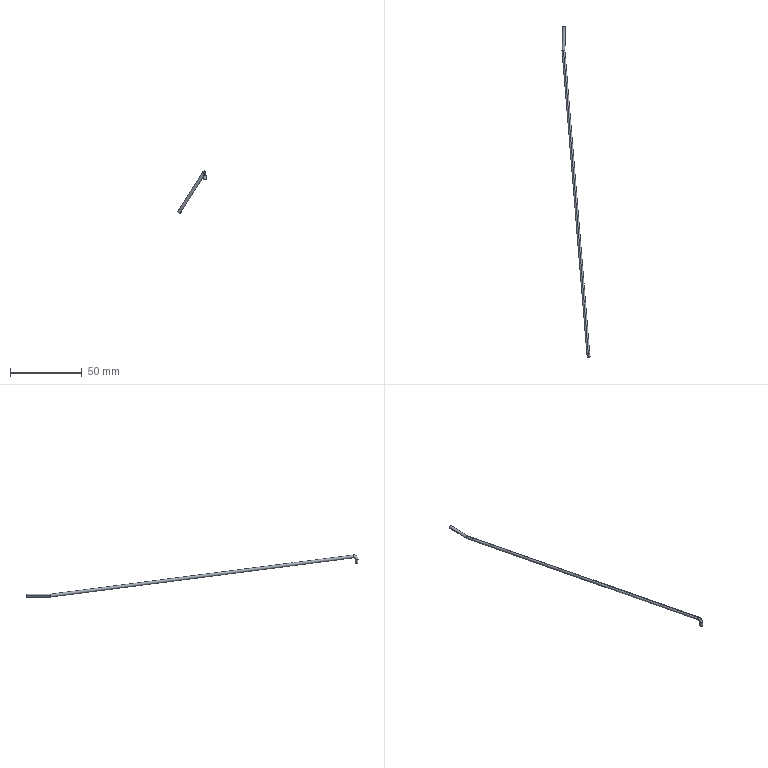Part | STEP file | rear_spoke4 | 1 solid | 10 faces | box 19.566 x 231.981 x 29.396 mm | volume 746.049 mm3 | cylinder 6 | torus 2 | plane 2 | commonest cylinder face diameters 2 x6
STEP:
#1=CARTESIAN_POINT('',(0.,0.,0.));
#2=DIRECTION('',(0.,0.,1.));
#3=DIRECTION('',(1.,0.,0.));
#4=AXIS2_PLACEMENT_3D('',#1,#2,#3);
#5=CARTESIAN_POINT('',(23.113,16.112,-0.1044));
#6=VERTEX_POINT('',#5);
#7=CARTESIAN_POINT('',(24.194,15.115,-0.1044));
#8=VERTEX_POINT('',#7);
#9=CARTESIAN_POINT('',(24.113,16.112,-0.1044));
#10=DIRECTION('',(0.,0.,1.));
#11=DIRECTION('',(1.,0.,0.));
#12=AXIS2_PLACEMENT_3D('',#9,#10,#11);
#13=CIRCLE('',#12,1.);
#14=CARTESIAN_POINT('',(23.949,18.105,-0.1044));
#15=DIRECTION('',(-0.9966,-0.08183,0.));
#16=DIRECTION('',(0.08183,-0.9966,0.));
#17=AXIS2_PLACEMENT_3D('',#14,#15,#16);
#18=TOROIDAL_SURFACE('',#17,2.,1.);
#19=CARTESIAN_POINT('',(0.,4.794));
#20=DIRECTION('',(0.,-1.));
#21=VECTOR('',#20,1.);
#22=LINE('',#19,#21);
#23=(GEOMETRIC_REPRESENTATION_CONTEXT(2)PARAMETRIC_REPRESENTATION_CONTEXT()REPRESENTATION_CONTEXT('',''));
#24=DEFINITIONAL_REPRESENTATION('',(#22),#23);
#25=PCURVE('',#18,#24);
#26=CARTESIAN_POINT('',(24.113,16.112,-3.));
#27=DIRECTION('',(0.,0.,1.));
#28=DIRECTION('',(1.,0.,0.));
#29=AXIS2_PLACEMENT_3D('',#26,#27,#28);
#30=CYLINDRICAL_SURFACE('',#29,1.);
#31=CARTESIAN_POINT('',(0.,2.896));
#32=DIRECTION('',(1.,0.));
#33=VECTOR('',#32,1.);
#34=LINE('',#31,#33);
#35=(GEOMETRIC_REPRESENTATION_CONTEXT(2)PARAMETRIC_REPRESENTATION_CONTEXT()REPRESENTATION_CONTEXT('',''));
#36=DEFINITIONAL_REPRESENTATION('',(#34),#35);
#37=PCURVE('',#30,#36);
#38=SURFACE_CURVE('',#13,(#25,#37),.PCURVE_S1.);
#39=EDGE_CURVE('',#6,#8,#38,.T.);
#40=ORIENTED_EDGE('',*,*,#39,.T.);
#41=CARTESIAN_POINT('',(23.918,18.487,2.871));
#42=VERTEX_POINT('',#41);
#43=CARTESIAN_POINT('',(23.949,18.105,-0.1044));
#44=DIRECTION('',(-0.9966,-0.08183,0.));
#45=DIRECTION('',(0.08183,-0.9966,0.));
#46=AXIS2_PLACEMENT_3D('',#43,#44,#45);
#47=CIRCLE('',#46,3.);
#48=CARTESIAN_POINT('',(0.,0.));
#49=DIRECTION('',(1.,0.));
#50=VECTOR('',#49,1.);
#51=LINE('',#48,#50);
#52=(GEOMETRIC_REPRESENTATION_CONTEXT(2)PARAMETRIC_REPRESENTATION_CONTEXT()REPRESENTATION_CONTEXT('',''));
#53=DEFINITIONAL_REPRESENTATION('',(#51),#52);
#54=PCURVE('',#18,#53);
#55=CARTESIAN_POINT('',(23.949,18.105,-0.1044));
#56=DIRECTION('',(-0.9966,-0.08183,0.));
#57=DIRECTION('',(0.08183,-0.9966,0.));
#58=AXIS2_PLACEMENT_3D('',#55,#56,#57);
#59=TOROIDAL_SURFACE('',#58,2.,1.);
#60=CARTESIAN_POINT('',(0.,6.283));
#61=DIRECTION('',(1.,0.));
#62=VECTOR('',#61,1.);
#63=LINE('',#60,#62);
#64=(GEOMETRIC_REPRESENTATION_CONTEXT(2)PARAMETRIC_REPRESENTATION_CONTEXT()REPRESENTATION_CONTEXT('',''));
#65=DEFINITIONAL_REPRESENTATION('',(#63),#64);
#66=PCURVE('',#59,#65);
#67=SURFACE_CURVE('',#47,(#54,#66),.PCURVE_S1.);
#68=EDGE_CURVE('',#8,#42,#67,.T.);
#69=ORIENTED_EDGE('',*,*,#68,.T.);
#70=CARTESIAN_POINT('',(23.928,18.231,0.8875));
#71=VERTEX_POINT('',#70);
#72=CARTESIAN_POINT('',(23.928,18.36,1.879));
#73=DIRECTION('',(-0.08116,0.9885,-0.1278));
#74=DIRECTION('',(0.9924,0.09198,0.08116));
#75=AXIS2_PLACEMENT_3D('',#72,#73,#74);
#76=CIRCLE('',#75,1.);
#77=CARTESIAN_POINT('',(1.699,4.794));
#78=DIRECTION('',(0.,-1.));
#79=VECTOR('',#78,1.);
#80=LINE('',#77,#79);
#81=(GEOMETRIC_REPRESENTATION_CONTEXT(2)PARAMETRIC_REPRESENTATION_CONTEXT()REPRESENTATION_CONTEXT('',''));
#82=DEFINITIONAL_REPRESENTATION('',(#80),#81);
#83=PCURVE('',#18,#82);
#84=CARTESIAN_POINT('',(23.928,18.36,1.879));
#85=DIRECTION('',(-0.08116,0.9885,-0.1278));
#86=DIRECTION('',(0.,0.1283,0.9917));
#87=AXIS2_PLACEMENT_3D('',#84,#85,#86);
#88=CYLINDRICAL_SURFACE('',#87,1.);
#89=CARTESIAN_POINT('',(1.478,0.));
#90=DIRECTION('',(1.,0.));
#91=VECTOR('',#90,1.);
#92=LINE('',#89,#91);
#93=(GEOMETRIC_REPRESENTATION_CONTEXT(2)PARAMETRIC_REPRESENTATION_CONTEXT()REPRESENTATION_CONTEXT('',''));
#94=DEFINITIONAL_REPRESENTATION('',(#92),#93);
#95=PCURVE('',#88,#94);
#96=SURFACE_CURVE('',#76,(#83,#95),.PCURVE_S1.);
#97=EDGE_CURVE('',#71,#42,#96,.T.);
#98=ORIENTED_EDGE('',*,*,#97,.F.);
#99=CARTESIAN_POINT('',(23.939,18.232,0.8874));
#100=VERTEX_POINT('',#99);
#101=CARTESIAN_POINT('',(23.928,18.36,1.879));
#102=DIRECTION('',(-0.08116,0.9885,-0.1278));
#103=DIRECTION('',(0.9924,0.09198,0.08116));
#104=AXIS2_PLACEMENT_3D('',#101,#102,#103);
#105=CIRCLE('',#104,1.);
#106=CARTESIAN_POINT('',(1.699,4.794));
#107=DIRECTION('',(0.,-1.));
#108=VECTOR('',#107,1.);
#109=LINE('',#106,#108);
#110=(GEOMETRIC_REPRESENTATION_CONTEXT(2)PARAMETRIC_REPRESENTATION_CONTEXT()REPRESENTATION_CONTEXT('',''));
#111=DEFINITIONAL_REPRESENTATION('',(#109),#110);
#112=PCURVE('',#18,#111);
#113=CARTESIAN_POINT('',(23.928,18.36,1.879));
#114=DIRECTION('',(-0.08116,0.9885,-0.1278));
#115=DIRECTION('',(0.,0.1283,0.9917));
#116=AXIS2_PLACEMENT_3D('',#113,#114,#115);
#117=CYLINDRICAL_SURFACE('',#116,1.);
#118=CARTESIAN_POINT('',(1.478,0.));
#119=DIRECTION('',(1.,0.));
#120=VECTOR('',#119,1.);
#121=LINE('',#118,#120);
#122=(GEOMETRIC_REPRESENTATION_CONTEXT(2)PARAMETRIC_REPRESENTATION_CONTEXT()REPRESENTATION_CONTEXT('',''));
#123=DEFINITIONAL_REPRESENTATION('',(#121),#122);
#124=PCURVE('',#117,#123);
#125=SURFACE_CURVE('',#105,(#112,#124),.PCURVE_S1.);
#126=EDGE_CURVE('',#100,#71,#125,.T.);
#127=ORIENTED_EDGE('',*,*,#126,.F.);
#128=CARTESIAN_POINT('',(24.031,17.108,-0.1044));
#129=VERTEX_POINT('',#128);
#130=CARTESIAN_POINT('',(23.949,18.105,-0.1044));
#131=DIRECTION('',(-0.9966,-0.08183,0.));
#132=DIRECTION('',(0.08183,-0.9966,0.));
#133=AXIS2_PLACEMENT_3D('',#130,#131,#132);
#134=CIRCLE('',#133,1.);
#135=CARTESIAN_POINT('',(0.,3.142));
#136=DIRECTION('',(1.,0.));
#137=VECTOR('',#136,1.);
#138=LINE('',#135,#137);
#139=(GEOMETRIC_REPRESENTATION_CONTEXT(2)PARAMETRIC_REPRESENTATION_CONTEXT()REPRESENTATION_CONTEXT('',''));
#140=DEFINITIONAL_REPRESENTATION('',(#138),#139);
#141=PCURVE('',#18,#140);
#142=CARTESIAN_POINT('',(0.,3.142));
#143=DIRECTION('',(1.,0.));
#144=VECTOR('',#143,1.);
#145=LINE('',#142,#144);
#146=(GEOMETRIC_REPRESENTATION_CONTEXT(2)PARAMETRIC_REPRESENTATION_CONTEXT()REPRESENTATION_CONTEXT('',''));
#147=DEFINITIONAL_REPRESENTATION('',(#145),#146);
#148=PCURVE('',#59,#147);
#149=SURFACE_CURVE('',#134,(#141,#148),.PCURVE_S1.);
#150=EDGE_CURVE('',#129,#100,#149,.T.);
#151=ORIENTED_EDGE('',*,*,#150,.F.);
#152=CARTESIAN_POINT('',(24.113,16.112,-0.1044));
#153=DIRECTION('',(0.,0.,1.));
#154=DIRECTION('',(1.,0.,0.));
#155=AXIS2_PLACEMENT_3D('',#152,#153,#154);
#156=CIRCLE('',#155,1.);
#157=CARTESIAN_POINT('',(0.,4.794));
#158=DIRECTION('',(0.,-1.));
#159=VECTOR('',#158,1.);
#160=LINE('',#157,#159);
#161=(GEOMETRIC_REPRESENTATION_CONTEXT(2)PARAMETRIC_REPRESENTATION_CONTEXT()REPRESENTATION_CONTEXT('',''));
#162=DEFINITIONAL_REPRESENTATION('',(#160),#161);
#163=PCURVE('',#18,#162);
#164=CARTESIAN_POINT('',(24.113,16.112,-3.));
#165=DIRECTION('',(0.,0.,1.));
#166=DIRECTION('',(1.,0.,0.));
#167=AXIS2_PLACEMENT_3D('',#164,#165,#166);
#168=CYLINDRICAL_SURFACE('',#167,1.);
#169=CARTESIAN_POINT('',(0.,2.896));
#170=DIRECTION('',(1.,0.));
#171=VECTOR('',#170,1.);
#172=LINE('',#169,#171);
#173=(GEOMETRIC_REPRESENTATION_CONTEXT(2)PARAMETRIC_REPRESENTATION_CONTEXT()REPRESENTATION_CONTEXT('',''));
#174=DEFINITIONAL_REPRESENTATION('',(#172),#173);
#175=PCURVE('',#168,#174);
#176=SURFACE_CURVE('',#156,(#163,#175),.PCURVE_S1.);
#177=EDGE_CURVE('',#129,#6,#176,.T.);
#178=ORIENTED_EDGE('',*,*,#177,.T.);
#179=EDGE_LOOP('',(#40,#69,#98,#127,#151,#178));
#180=FACE_BOUND('',#179,.T.);
#181=ADVANCED_FACE('',(#180),#18,.T.);
#182=CARTESIAN_POINT('',(23.928,18.488,2.871));
#183=VERTEX_POINT('',#182);
#184=CARTESIAN_POINT('',(23.928,18.36,1.879));
#185=DIRECTION('',(-0.08116,0.9885,-0.1278));
#186=DIRECTION('',(0.9924,0.09198,0.08116));
#187=AXIS2_PLACEMENT_3D('',#184,#185,#186);
#188=CIRCLE('',#187,1.);
#189=CARTESIAN_POINT('',(-4.805,0.));
#190=DIRECTION('',(1.,0.));
#191=VECTOR('',#190,1.);
#192=LINE('',#189,#191);
#193=(GEOMETRIC_REPRESENTATION_CONTEXT(2)PARAMETRIC_REPRESENTATION_CONTEXT()REPRESENTATION_CONTEXT('',''));
#194=DEFINITIONAL_REPRESENTATION('',(#192),#193);
#195=PCURVE('',#117,#194);
#196=CARTESIAN_POINT('',(1.699,11.077));
#197=DIRECTION('',(0.,-1.));
#198=VECTOR('',#197,1.);
#199=LINE('',#196,#198);
#200=(GEOMETRIC_REPRESENTATION_CONTEXT(2)PARAMETRIC_REPRESENTATION_CONTEXT()REPRESENTATION_CONTEXT('',''));
#201=DEFINITIONAL_REPRESENTATION('',(#199),#200);
#202=PCURVE('',#59,#201);
#203=SURFACE_CURVE('',#188,(#195,#202),.PCURVE_S1.);
#204=EDGE_CURVE('',#183,#100,#203,.T.);
#205=ORIENTED_EDGE('',*,*,#204,.T.);
#206=ORIENTED_EDGE('',*,*,#126,.T.);
#207=CARTESIAN_POINT('',(6.542,229.983,-26.5));
#208=VERTEX_POINT('',#207);
#209=CARTESIAN_POINT('',(23.928,18.231,0.8875));
#210=DIRECTION('',(-0.08116,0.9885,-0.1278));
#211=VECTOR('',#210,1.);
#212=LINE('',#209,#211);
#213=CARTESIAN_POINT('',(3.142,0.));
#214=DIRECTION('',(0.,1.));
#215=VECTOR('',#214,1.);
#216=LINE('',#213,#215);
#217=(GEOMETRIC_REPRESENTATION_CONTEXT(2)PARAMETRIC_REPRESENTATION_CONTEXT()REPRESENTATION_CONTEXT('',''));
#218=DEFINITIONAL_REPRESENTATION('',(#216),#217);
#219=PCURVE('',#117,#218);
#220=CARTESIAN_POINT('',(3.142,0.));
#221=DIRECTION('',(0.,1.));
#222=VECTOR('',#221,1.);
#223=LINE('',#220,#222);
#224=(GEOMETRIC_REPRESENTATION_CONTEXT(2)PARAMETRIC_REPRESENTATION_CONTEXT()REPRESENTATION_CONTEXT('',''));
#225=DEFINITIONAL_REPRESENTATION('',(#223),#224);
#226=PCURVE('',#88,#225);
#227=SURFACE_CURVE('',#212,(#219,#226),.PCURVE_S1.);
#228=EDGE_CURVE('',#71,#208,#227,.T.);
#229=ORIENTED_EDGE('',*,*,#228,.T.);
#230=CARTESIAN_POINT('',(7.549,230.074,-25.5));
#231=VERTEX_POINT('',#230);
#232=CARTESIAN_POINT('',(6.542,229.983,-26.5));
#233=CARTESIAN_POINT('',(7.131,229.998,-26.502));
#234=CARTESIAN_POINT('',(7.548,230.036,-26.087));
#235=CARTESIAN_POINT('',(7.549,230.074,-25.5));
#236=(BOUNDED_CURVE()B_SPLINE_CURVE(3,(#232,#233,#234,#235),.UNSPECIFIED.,.F.,.F.)B_SPLINE_CURVE_WITH_KNOTS((4,4),(0.7037,2.278),.PIECEWISE_BEZIER_KNOTS.)CURVE()GEOMETRIC_REPRESENTATION_ITEM()RATIONAL_B_SPLINE_CURVE((1.,0.8039,0.8039,1.))REPRESENTATION_ITEM(''));
#237=CARTESIAN_POINT('',(3.142,214.222));
#238=CARTESIAN_POINT('',(3.12,214.221));
#239=CARTESIAN_POINT('',(3.077,214.218));
#240=CARTESIAN_POINT('',(3.01,214.214));
#241=CARTESIAN_POINT('',(2.941,214.21));
#242=CARTESIAN_POINT('',(2.871,214.205));
#243=CARTESIAN_POINT('',(2.8,214.2));
#244=CARTESIAN_POINT('',(2.728,214.195));
#245=CARTESIAN_POINT('',(2.654,214.189));
#246=CARTESIAN_POINT('',(2.58,214.183));
#247=CARTESIAN_POINT('',(2.505,214.177));
#248=CARTESIAN_POINT('',(2.43,214.171));
#249=CARTESIAN_POINT('',(2.354,214.164));
#250=CARTESIAN_POINT('',(2.279,214.158));
#251=CARTESIAN_POINT('',(2.204,214.151));
#252=CARTESIAN_POINT('',(2.129,214.145));
#253=CARTESIAN_POINT('',(2.055,214.139));
#254=CARTESIAN_POINT('',(1.981,214.133));
#255=CARTESIAN_POINT('',(1.909,214.127));
#256=CARTESIAN_POINT('',(1.838,214.122));
#257=CARTESIAN_POINT('',(1.768,214.116));
#258=CARTESIAN_POINT('',(1.699,214.111));
#259=CARTESIAN_POINT('',(1.632,214.107));
#260=CARTESIAN_POINT('',(1.589,214.104));
#261=CARTESIAN_POINT('',(1.567,214.102));
#262=B_SPLINE_CURVE_WITH_KNOTS('',3,(#237,#238,#239,#240,#241,#242,#243,#244,#245,#246,#247,#248,#249,#250,#251,#252,#253,#254,#255,#256,#257,#258,#259,#260,#261),.UNSPECIFIED.,.F.,.F.,(4,1,1,1,1,1,1,1,1,1,1,1,1,1,1,1,1,1,1,1,1,1,4),(0.7037,0.7753,0.8468,0.9184,0.9899,1.061,1.133,1.205,1.276,1.348,1.419,1.491,1.562,1.634,1.705,1.777,1.849,1.92,1.992,2.063,2.135,2.206,2.278),.QUASI_UNIFORM_KNOTS.);
#263=(GEOMETRIC_REPRESENTATION_CONTEXT(2)PARAMETRIC_REPRESENTATION_CONTEXT()REPRESENTATION_CONTEXT('',''));
#264=DEFINITIONAL_REPRESENTATION('',(#262),#263);
#265=PCURVE('',#117,#264);
#266=CARTESIAN_POINT('',(6.539,229.751,-25.5));
#267=DIRECTION('',(0.02845,0.9996,0.));
#268=DIRECTION('',(-0.9996,0.02845,0.));
#269=AXIS2_PLACEMENT_3D('',#266,#267,#268);
#270=CYLINDRICAL_SURFACE('',#269,1.);
#271=CARTESIAN_POINT('',(4.716,0.2323));
#272=CARTESIAN_POINT('',(4.694,0.2335));
#273=CARTESIAN_POINT('',(4.651,0.236));
#274=CARTESIAN_POINT('',(4.584,0.24));
#275=CARTESIAN_POINT('',(4.515,0.2445));
#276=CARTESIAN_POINT('',(4.446,0.2493));
#277=CARTESIAN_POINT('',(4.374,0.2544));
#278=CARTESIAN_POINT('',(4.302,0.2598));
#279=CARTESIAN_POINT('',(4.229,0.2655));
#280=CARTESIAN_POINT('',(4.154,0.2714));
#281=CARTESIAN_POINT('',(4.079,0.2775));
#282=CARTESIAN_POINT('',(4.004,0.2838));
#283=CARTESIAN_POINT('',(3.929,0.2901));
#284=CARTESIAN_POINT('',(3.853,0.2965));
#285=CARTESIAN_POINT('',(3.778,0.3029));
#286=CARTESIAN_POINT('',(3.703,0.3092));
#287=CARTESIAN_POINT('',(3.629,0.3154));
#288=CARTESIAN_POINT('',(3.555,0.3214));
#289=CARTESIAN_POINT('',(3.483,0.3272));
#290=CARTESIAN_POINT('',(3.412,0.3328));
#291=CARTESIAN_POINT('',(3.342,0.338));
#292=CARTESIAN_POINT('',(3.273,0.343));
#293=CARTESIAN_POINT('',(3.207,0.3476));
#294=CARTESIAN_POINT('',(3.163,0.3505));
#295=CARTESIAN_POINT('',(3.142,0.3519));
#296=B_SPLINE_CURVE_WITH_KNOTS('',3,(#271,#272,#273,#274,#275,#276,#277,#278,#279,#280,#281,#282,#283,#284,#285,#286,#287,#288,#289,#290,#291,#292,#293,#294,#295),.UNSPECIFIED.,.F.,.F.,(4,1,1,1,1,1,1,1,1,1,1,1,1,1,1,1,1,1,1,1,1,1,4),(0.7037,0.7753,0.8468,0.9184,0.9899,1.061,1.133,1.205,1.276,1.348,1.419,1.491,1.562,1.634,1.705,1.777,1.849,1.92,1.992,2.063,2.135,2.206,2.278),.QUASI_UNIFORM_KNOTS.);
#297=(GEOMETRIC_REPRESENTATION_CONTEXT(2)PARAMETRIC_REPRESENTATION_CONTEXT()REPRESENTATION_CONTEXT('',''));
#298=DEFINITIONAL_REPRESENTATION('',(#296),#297);
#299=PCURVE('',#270,#298);
#300=SURFACE_CURVE('',#236,(#265,#299),.PCURVE_S1.);
#301=EDGE_CURVE('',#208,#231,#300,.T.);
#302=ORIENTED_EDGE('',*,*,#301,.T.);
#303=CARTESIAN_POINT('',(6.553,230.112,-24.5));
#304=VERTEX_POINT('',#303);
#305=CARTESIAN_POINT('',(7.549,230.074,-25.5));
#306=CARTESIAN_POINT('',(7.55,230.112,-24.916));
#307=CARTESIAN_POINT('',(7.138,230.127,-24.502));
#308=CARTESIAN_POINT('',(6.553,230.112,-24.5));
#309=(BOUNDED_CURVE()B_SPLINE_CURVE(3,(#305,#306,#307,#308),.UNSPECIFIED.,.F.,.F.)B_SPLINE_CURVE_WITH_KNOTS((4,4),(2.278,3.845),.PIECEWISE_BEZIER_KNOTS.)CURVE()GEOMETRIC_REPRESENTATION_ITEM()RATIONAL_B_SPLINE_CURVE((1.,0.8055,0.8055,1.))REPRESENTATION_ITEM(''));
#310=CARTESIAN_POINT('',(1.567,214.102));
#311=CARTESIAN_POINT('',(1.546,214.101));
#312=CARTESIAN_POINT('',(1.503,214.098));
#313=CARTESIAN_POINT('',(1.436,214.094));
#314=CARTESIAN_POINT('',(1.368,214.091));
#315=CARTESIAN_POINT('',(1.298,214.087));
#316=CARTESIAN_POINT('',(1.227,214.084));
#317=CARTESIAN_POINT('',(1.155,214.081));
#318=CARTESIAN_POINT('',(1.082,214.079));
#319=CARTESIAN_POINT('',(1.008,214.077));
#320=CARTESIAN_POINT('',(0.9337,214.075));
#321=CARTESIAN_POINT('',(0.8588,214.074));
#322=CARTESIAN_POINT('',(0.7837,214.073));
#323=CARTESIAN_POINT('',(0.7086,214.073));
#324=CARTESIAN_POINT('',(0.6336,214.073));
#325=CARTESIAN_POINT('',(0.5591,214.074));
#326=CARTESIAN_POINT('',(0.4853,214.075));
#327=CARTESIAN_POINT('',(0.4122,214.076));
#328=CARTESIAN_POINT('',(0.3401,214.078));
#329=CARTESIAN_POINT('',(0.2692,214.081));
#330=CARTESIAN_POINT('',(0.1996,214.083));
#331=CARTESIAN_POINT('',(0.1314,214.086));
#332=CARTESIAN_POINT('',(0.06474,214.089));
#333=CARTESIAN_POINT('',(0.02139,214.092));
#334=CARTESIAN_POINT('',(0.,214.093));
#335=B_SPLINE_CURVE_WITH_KNOTS('',3,(#310,#311,#312,#313,#314,#315,#316,#317,#318,#319,#320,#321,#322,#323,#324,#325,#326,#327,#328,#329,#330,#331,#332,#333,#334),.UNSPECIFIED.,.F.,.F.,(4,1,1,1,1,1,1,1,1,1,1,1,1,1,1,1,1,1,1,1,1,1,4),(2.278,2.349,2.42,2.492,2.563,2.634,2.705,2.777,2.848,2.919,2.99,3.062,3.133,3.204,3.275,3.347,3.418,3.489,3.56,3.632,3.703,3.774,3.845),.QUASI_UNIFORM_KNOTS.);
#336=(GEOMETRIC_REPRESENTATION_CONTEXT(2)PARAMETRIC_REPRESENTATION_CONTEXT()REPRESENTATION_CONTEXT('',''));
#337=DEFINITIONAL_REPRESENTATION('',(#335),#336);
#338=PCURVE('',#117,#337);
#339=CARTESIAN_POINT('',(6.539,229.751,-25.5));
#340=DIRECTION('',(0.02845,0.9996,0.));
#341=DIRECTION('',(-0.9996,0.02845,0.));
#342=AXIS2_PLACEMENT_3D('',#339,#340,#341);
#343=CYLINDRICAL_SURFACE('',#342,1.);
#344=CARTESIAN_POINT('',(3.142,0.3519));
#345=CARTESIAN_POINT('',(3.12,0.3533));
#346=CARTESIAN_POINT('',(3.077,0.356));
#347=CARTESIAN_POINT('',(3.01,0.3599));
#348=CARTESIAN_POINT('',(2.942,0.3636));
#349=CARTESIAN_POINT('',(2.872,0.3671));
#350=CARTESIAN_POINT('',(2.801,0.3703));
#351=CARTESIAN_POINT('',(2.729,0.3732));
#352=CARTESIAN_POINT('',(2.656,0.3757));
#353=CARTESIAN_POINT('',(2.582,0.3778));
#354=CARTESIAN_POINT('',(2.508,0.3794));
#355=CARTESIAN_POINT('',(2.433,0.3806));
#356=CARTESIAN_POINT('',(2.358,0.3814));
#357=CARTESIAN_POINT('',(2.283,0.3817));
#358=CARTESIAN_POINT('',(2.208,0.3814));
#359=CARTESIAN_POINT('',(2.133,0.3808));
#360=CARTESIAN_POINT('',(2.059,0.3796));
#361=CARTESIAN_POINT('',(1.986,0.3781));
#362=CARTESIAN_POINT('',(1.914,0.3761));
#363=CARTESIAN_POINT('',(1.843,0.3738));
#364=CARTESIAN_POINT('',(1.774,0.3711));
#365=CARTESIAN_POINT('',(1.706,0.3681));
#366=CARTESIAN_POINT('',(1.639,0.3649));
#367=CARTESIAN_POINT('',(1.596,0.3626));
#368=CARTESIAN_POINT('',(1.574,0.3615));
#369=B_SPLINE_CURVE_WITH_KNOTS('',3,(#344,#345,#346,#347,#348,#349,#350,#351,#352,#353,#354,#355,#356,#357,#358,#359,#360,#361,#362,#363,#364,#365,#366,#367,#368),.UNSPECIFIED.,.F.,.F.,(4,1,1,1,1,1,1,1,1,1,1,1,1,1,1,1,1,1,1,1,1,1,4),(2.278,2.349,2.42,2.492,2.563,2.634,2.705,2.777,2.848,2.919,2.99,3.062,3.133,3.204,3.275,3.347,3.418,3.489,3.56,3.632,3.703,3.774,3.845),.QUASI_UNIFORM_KNOTS.);
#370=(GEOMETRIC_REPRESENTATION_CONTEXT(2)PARAMETRIC_REPRESENTATION_CONTEXT()REPRESENTATION_CONTEXT('',''));
#371=DEFINITIONAL_REPRESENTATION('',(#369),#370);
#372=PCURVE('',#343,#371);
#373=SURFACE_CURVE('',#309,(#338,#372),.PCURVE_S1.);
#374=EDGE_CURVE('',#231,#304,#373,.T.);
#375=ORIENTED_EDGE('',*,*,#374,.T.);
#376=CARTESIAN_POINT('',(23.928,18.488,2.871));
#377=DIRECTION('',(-0.08116,0.9885,-0.1278));
#378=VECTOR('',#377,1.);
#379=LINE('',#376,#378);
#380=CARTESIAN_POINT('',(0.,0.));
#381=DIRECTION('',(0.,1.));
#382=VECTOR('',#381,1.);
#383=LINE('',#380,#382);
#384=(GEOMETRIC_REPRESENTATION_CONTEXT(2)PARAMETRIC_REPRESENTATION_CONTEXT()REPRESENTATION_CONTEXT('',''));
#385=DEFINITIONAL_REPRESENTATION('',(#383),#384);
#386=PCURVE('',#117,#385);
#387=CARTESIAN_POINT('',(6.283,0.));
#388=DIRECTION('',(0.,1.));
#389=VECTOR('',#388,1.);
#390=LINE('',#387,#389);
#391=(GEOMETRIC_REPRESENTATION_CONTEXT(2)PARAMETRIC_REPRESENTATION_CONTEXT()REPRESENTATION_CONTEXT('',''));
#392=DEFINITIONAL_REPRESENTATION('',(#390),#391);
#393=PCURVE('',#88,#392);
#394=SURFACE_CURVE('',#379,(#386,#393),.PCURVE_S1.);
#395=EDGE_CURVE('',#183,#304,#394,.T.);
#396=ORIENTED_EDGE('',*,*,#395,.F.);
#397=EDGE_LOOP('',(#205,#206,#229,#302,#375,#396));
#398=FACE_BOUND('',#397,.T.);
#399=ADVANCED_FACE('',(#398),#117,.T.);
#400=CARTESIAN_POINT('',(25.113,16.112,-3.));
#401=VERTEX_POINT('',#400);
#402=CARTESIAN_POINT('',(23.113,16.112,-3.));
#403=VERTEX_POINT('',#402);
#404=CARTESIAN_POINT('',(24.113,16.112,-3.));
#405=DIRECTION('',(0.,0.,1.));
#406=DIRECTION('',(1.,0.,0.));
#407=AXIS2_PLACEMENT_3D('',#404,#405,#406);
#408=CIRCLE('',#407,1.);
#409=CARTESIAN_POINT('',(0.,0.));
#410=DIRECTION('',(1.,0.));
#411=VECTOR('',#410,1.);
#412=LINE('',#409,#411);
#413=(GEOMETRIC_REPRESENTATION_CONTEXT(2)PARAMETRIC_REPRESENTATION_CONTEXT()REPRESENTATION_CONTEXT('',''));
#414=DEFINITIONAL_REPRESENTATION('',(#412),#413);
#415=PCURVE('',#168,#414);
#416=CARTESIAN_POINT('',(24.113,16.112,-3.));
#417=DIRECTION('',(0.,0.,1.));
#418=DIRECTION('',(1.,0.,0.));
#419=AXIS2_PLACEMENT_3D('',#416,#417,#418);
#420=PLANE('',#419);
#421=CARTESIAN_POINT('',(0.,0.));
#422=DIRECTION('',(1.,0.));
#423=AXIS2_PLACEMENT_2D('',#421,#422);
#424=CIRCLE('',#423,1.);
#425=(GEOMETRIC_REPRESENTATION_CONTEXT(2)PARAMETRIC_REPRESENTATION_CONTEXT()REPRESENTATION_CONTEXT('',''));
#426=DEFINITIONAL_REPRESENTATION('',(#424),#425);
#427=PCURVE('',#420,#426);
#428=SURFACE_CURVE('',#408,(#415,#427),.PCURVE_S1.);
#429=EDGE_CURVE('',#401,#403,#428,.T.);
#430=ORIENTED_EDGE('',*,*,#429,.T.);
#431=CARTESIAN_POINT('',(23.113,16.112,-3.));
#432=DIRECTION('',(0.,0.,1.));
#433=VECTOR('',#432,1.);
#434=LINE('',#431,#433);
#435=CARTESIAN_POINT('',(3.142,0.));
#436=DIRECTION('',(0.,1.));
#437=VECTOR('',#436,1.);
#438=LINE('',#435,#437);
#439=(GEOMETRIC_REPRESENTATION_CONTEXT(2)PARAMETRIC_REPRESENTATION_CONTEXT()REPRESENTATION_CONTEXT('',''));
#440=DEFINITIONAL_REPRESENTATION('',(#438),#439);
#441=PCURVE('',#168,#440);
#442=CARTESIAN_POINT('',(3.142,0.));
#443=DIRECTION('',(0.,1.));
#444=VECTOR('',#443,1.);
#445=LINE('',#442,#444);
#446=(GEOMETRIC_REPRESENTATION_CONTEXT(2)PARAMETRIC_REPRESENTATION_CONTEXT()REPRESENTATION_CONTEXT('',''));
#447=DEFINITIONAL_REPRESENTATION('',(#445),#446);
#448=PCURVE('',#30,#447);
#449=SURFACE_CURVE('',#434,(#441,#448),.PCURVE_S1.);
#450=EDGE_CURVE('',#403,#6,#449,.T.);
#451=ORIENTED_EDGE('',*,*,#450,.T.);
#452=ORIENTED_EDGE('',*,*,#177,.F.);
#453=CARTESIAN_POINT('',(25.113,16.112,-0.1044));
#454=VERTEX_POINT('',#453);
#455=CARTESIAN_POINT('',(24.113,16.112,-0.1044));
#456=DIRECTION('',(0.,0.,1.));
#457=DIRECTION('',(1.,0.,0.));
#458=AXIS2_PLACEMENT_3D('',#455,#456,#457);
#459=CIRCLE('',#458,1.);
#460=CARTESIAN_POINT('',(0.,2.896));
#461=DIRECTION('',(1.,0.));
#462=VECTOR('',#461,1.);
#463=LINE('',#460,#462);
#464=(GEOMETRIC_REPRESENTATION_CONTEXT(2)PARAMETRIC_REPRESENTATION_CONTEXT()REPRESENTATION_CONTEXT('',''));
#465=DEFINITIONAL_REPRESENTATION('',(#463),#464);
#466=PCURVE('',#168,#465);
#467=CARTESIAN_POINT('',(0.,4.794));
#468=DIRECTION('',(0.,-1.));
#469=VECTOR('',#468,1.);
#470=LINE('',#467,#469);
#471=(GEOMETRIC_REPRESENTATION_CONTEXT(2)PARAMETRIC_REPRESENTATION_CONTEXT()REPRESENTATION_CONTEXT('',''));
#472=DEFINITIONAL_REPRESENTATION('',(#470),#471);
#473=PCURVE('',#59,#472);
#474=SURFACE_CURVE('',#459,(#466,#473),.PCURVE_S1.);
#475=EDGE_CURVE('',#454,#129,#474,.T.);
#476=ORIENTED_EDGE('',*,*,#475,.F.);
#477=CARTESIAN_POINT('',(25.113,16.112,-3.));
#478=DIRECTION('',(0.,0.,1.));
#479=VECTOR('',#478,1.);
#480=LINE('',#477,#479);
#481=CARTESIAN_POINT('',(0.,0.));
#482=DIRECTION('',(0.,1.));
#483=VECTOR('',#482,1.);
#484=LINE('',#481,#483);
#485=(GEOMETRIC_REPRESENTATION_CONTEXT(2)PARAMETRIC_REPRESENTATION_CONTEXT()REPRESENTATION_CONTEXT('',''));
#486=DEFINITIONAL_REPRESENTATION('',(#484),#485);
#487=PCURVE('',#168,#486);
#488=CARTESIAN_POINT('',(6.283,0.));
#489=DIRECTION('',(0.,1.));
#490=VECTOR('',#489,1.);
#491=LINE('',#488,#490);
#492=(GEOMETRIC_REPRESENTATION_CONTEXT(2)PARAMETRIC_REPRESENTATION_CONTEXT()REPRESENTATION_CONTEXT('',''));
#493=DEFINITIONAL_REPRESENTATION('',(#491),#492);
#494=PCURVE('',#30,#493);
#495=SURFACE_CURVE('',#480,(#487,#494),.PCURVE_S1.);
#496=EDGE_CURVE('',#401,#454,#495,.T.);
#497=ORIENTED_EDGE('',*,*,#496,.F.);
#498=EDGE_LOOP('',(#430,#451,#452,#476,#497));
#499=FACE_BOUND('',#498,.T.);
#500=ADVANCED_FACE('',(#499),#168,.T.);
#501=ORIENTED_EDGE('',*,*,#374,.F.);
#502=CARTESIAN_POINT('',(8.032,247.036,-25.5));
#503=VERTEX_POINT('',#502);
#504=CARTESIAN_POINT('',(7.539,229.722,-25.5));
#505=DIRECTION('',(0.02845,0.9996,0.));
#506=VECTOR('',#505,1.);
#507=LINE('',#504,#506);
#508=CARTESIAN_POINT('',(3.142,0.));
#509=DIRECTION('',(0.,1.));
#510=VECTOR('',#509,1.);
#511=LINE('',#508,#510);
#512=(GEOMETRIC_REPRESENTATION_CONTEXT(2)PARAMETRIC_REPRESENTATION_CONTEXT()REPRESENTATION_CONTEXT('',''));
#513=DEFINITIONAL_REPRESENTATION('',(#511),#512);
#514=PCURVE('',#343,#513);
#515=CARTESIAN_POINT('',(3.142,0.));
#516=DIRECTION('',(0.,1.));
#517=VECTOR('',#516,1.);
#518=LINE('',#515,#517);
#519=(GEOMETRIC_REPRESENTATION_CONTEXT(2)PARAMETRIC_REPRESENTATION_CONTEXT()REPRESENTATION_CONTEXT('',''));
#520=DEFINITIONAL_REPRESENTATION('',(#518),#519);
#521=PCURVE('',#270,#520);
#522=SURFACE_CURVE('',#507,(#514,#521),.PCURVE_S1.);
#523=EDGE_CURVE('',#231,#503,#522,.T.);
#524=ORIENTED_EDGE('',*,*,#523,.T.);
#525=CARTESIAN_POINT('',(6.032,247.093,-25.5));
#526=VERTEX_POINT('',#525);
#527=CARTESIAN_POINT('',(7.032,247.064,-25.5));
#528=DIRECTION('',(0.02845,0.9996,0.));
#529=DIRECTION('',(0.9956,-0.02834,0.08889));
#530=AXIS2_PLACEMENT_3D('',#527,#528,#529);
#531=CIRCLE('',#530,1.);
#532=CARTESIAN_POINT('',(-3.231,17.321));
#533=DIRECTION('',(1.,0.));
#534=VECTOR('',#533,1.);
#535=LINE('',#532,#534);
#536=(GEOMETRIC_REPRESENTATION_CONTEXT(2)PARAMETRIC_REPRESENTATION_CONTEXT()REPRESENTATION_CONTEXT('',''));
#537=DEFINITIONAL_REPRESENTATION('',(#535),#536);
#538=PCURVE('',#343,#537);
#539=CARTESIAN_POINT('',(7.032,247.064,-25.5));
#540=DIRECTION('',(0.02845,0.9996,0.));
#541=DIRECTION('',(0.9956,-0.02834,0.08889));
#542=AXIS2_PLACEMENT_3D('',#539,#540,#541);
#543=PLANE('',#542);
#544=CARTESIAN_POINT('',(0.,0.));
#545=DIRECTION('',(1.,0.));
#546=AXIS2_PLACEMENT_2D('',#544,#545);
#547=CIRCLE('',#546,1.);
#548=(GEOMETRIC_REPRESENTATION_CONTEXT(2)PARAMETRIC_REPRESENTATION_CONTEXT()REPRESENTATION_CONTEXT('',''));
#549=DEFINITIONAL_REPRESENTATION('',(#547),#548);
#550=PCURVE('',#543,#549);
#551=SURFACE_CURVE('',#531,(#538,#550),.PCURVE_S1.);
#552=EDGE_CURVE('',#526,#503,#551,.T.);
#553=ORIENTED_EDGE('',*,*,#552,.F.);
#554=CARTESIAN_POINT('',(5.547,230.021,-25.5));
#555=VERTEX_POINT('',#554);
#556=CARTESIAN_POINT('',(5.54,229.779,-25.5));
#557=DIRECTION('',(0.02845,0.9996,0.));
#558=VECTOR('',#557,1.);
#559=LINE('',#556,#558);
#560=CARTESIAN_POINT('',(0.,0.));
#561=DIRECTION('',(0.,1.));
#562=VECTOR('',#561,1.);
#563=LINE('',#560,#562);
#564=(GEOMETRIC_REPRESENTATION_CONTEXT(2)PARAMETRIC_REPRESENTATION_CONTEXT()REPRESENTATION_CONTEXT('',''));
#565=DEFINITIONAL_REPRESENTATION('',(#563),#564);
#566=PCURVE('',#343,#565);
#567=CARTESIAN_POINT('',(6.283,0.));
#568=DIRECTION('',(0.,1.));
#569=VECTOR('',#568,1.);
#570=LINE('',#567,#569);
#571=(GEOMETRIC_REPRESENTATION_CONTEXT(2)PARAMETRIC_REPRESENTATION_CONTEXT()REPRESENTATION_CONTEXT('',''));
#572=DEFINITIONAL_REPRESENTATION('',(#570),#571);
#573=PCURVE('',#270,#572);
#574=SURFACE_CURVE('',#559,(#566,#573),.PCURVE_S1.);
#575=EDGE_CURVE('',#555,#526,#574,.T.);
#576=ORIENTED_EDGE('',*,*,#575,.F.);
#577=CARTESIAN_POINT('',(6.553,230.112,-24.5));
#578=CARTESIAN_POINT('',(5.965,230.096,-24.498));
#579=CARTESIAN_POINT('',(5.548,230.059,-24.913));
#580=CARTESIAN_POINT('',(5.547,230.021,-25.5));
#581=(BOUNDED_CURVE()B_SPLINE_CURVE(3,(#577,#578,#579,#580),.UNSPECIFIED.,.F.,.F.)B_SPLINE_CURVE_WITH_KNOTS((4,4),(3.845,5.419),.PIECEWISE_BEZIER_KNOTS.)CURVE()GEOMETRIC_REPRESENTATION_ITEM()RATIONAL_B_SPLINE_CURVE((1.,0.8039,0.8039,1.))REPRESENTATION_ITEM(''));
#582=CARTESIAN_POINT('',(1.574,0.3615));
#583=CARTESIAN_POINT('',(1.553,0.3603));
#584=CARTESIAN_POINT('',(1.509,0.3578));
#585=CARTESIAN_POINT('',(1.442,0.3537));
#586=CARTESIAN_POINT('',(1.374,0.3493));
#587=CARTESIAN_POINT('',(1.304,0.3445));
#588=CARTESIAN_POINT('',(1.233,0.3394));
#589=CARTESIAN_POINT('',(1.16,0.334));
#590=CARTESIAN_POINT('',(1.087,0.3283));
#591=CARTESIAN_POINT('',(1.013,0.3224));
#592=CARTESIAN_POINT('',(0.9379,0.3163));
#593=CARTESIAN_POINT('',(0.8626,0.31));
#594=CARTESIAN_POINT('',(0.7871,0.3037));
#595=CARTESIAN_POINT('',(0.7116,0.2973));
#596=CARTESIAN_POINT('',(0.6363,0.2909));
#597=CARTESIAN_POINT('',(0.5615,0.2846));
#598=CARTESIAN_POINT('',(0.4873,0.2784));
#599=CARTESIAN_POINT('',(0.4139,0.2724));
#600=CARTESIAN_POINT('',(0.3415,0.2666));
#601=CARTESIAN_POINT('',(0.2702,0.261));
#602=CARTESIAN_POINT('',(0.2003,0.2558));
#603=CARTESIAN_POINT('',(0.1319,0.2508));
#604=CARTESIAN_POINT('',(0.06497,0.2461));
#605=CARTESIAN_POINT('',(0.02146,0.2433));
#606=CARTESIAN_POINT('',(0.,0.2419));
#607=B_SPLINE_CURVE_WITH_KNOTS('',3,(#582,#583,#584,#585,#586,#587,#588,#589,#590,#591,#592,#593,#594,#595,#596,#597,#598,#599,#600,#601,#602,#603,#604,#605,#606),.UNSPECIFIED.,.F.,.F.,(4,1,1,1,1,1,1,1,1,1,1,1,1,1,1,1,1,1,1,1,1,1,4),(3.845,3.917,3.988,4.06,4.132,4.203,4.275,4.346,4.418,4.489,4.561,4.632,4.704,4.776,4.847,4.919,4.99,5.062,5.133,5.205,5.276,5.348,5.419),.QUASI_UNIFORM_KNOTS.);
#608=(GEOMETRIC_REPRESENTATION_CONTEXT(2)PARAMETRIC_REPRESENTATION_CONTEXT()REPRESENTATION_CONTEXT('',''));
#609=DEFINITIONAL_REPRESENTATION('',(#607),#608);
#610=PCURVE('',#343,#609);
#611=CARTESIAN_POINT('',(6.283,214.093));
#612=CARTESIAN_POINT('',(6.262,214.094));
#613=CARTESIAN_POINT('',(6.218,214.096));
#614=CARTESIAN_POINT('',(6.151,214.101));
#615=CARTESIAN_POINT('',(6.083,214.105));
#616=CARTESIAN_POINT('',(6.013,214.11));
#617=CARTESIAN_POINT('',(5.942,214.115));
#618=CARTESIAN_POINT('',(5.869,214.12));
#619=CARTESIAN_POINT('',(5.796,214.126));
#620=CARTESIAN_POINT('',(5.722,214.132));
#621=CARTESIAN_POINT('',(5.647,214.138));
#622=CARTESIAN_POINT('',(5.572,214.144));
#623=CARTESIAN_POINT('',(5.496,214.151));
#624=CARTESIAN_POINT('',(5.421,214.157));
#625=CARTESIAN_POINT('',(5.345,214.163));
#626=CARTESIAN_POINT('',(5.27,214.17));
#627=CARTESIAN_POINT('',(5.196,214.176));
#628=CARTESIAN_POINT('',(5.123,214.182));
#629=CARTESIAN_POINT('',(5.05,214.188));
#630=CARTESIAN_POINT('',(4.979,214.193));
#631=CARTESIAN_POINT('',(4.909,214.199));
#632=CARTESIAN_POINT('',(4.841,214.204));
#633=CARTESIAN_POINT('',(4.774,214.208));
#634=CARTESIAN_POINT('',(4.73,214.211));
#635=CARTESIAN_POINT('',(4.709,214.212));
#636=B_SPLINE_CURVE_WITH_KNOTS('',3,(#611,#612,#613,#614,#615,#616,#617,#618,#619,#620,#621,#622,#623,#624,#625,#626,#627,#628,#629,#630,#631,#632,#633,#634,#635),.UNSPECIFIED.,.F.,.F.,(4,1,1,1,1,1,1,1,1,1,1,1,1,1,1,1,1,1,1,1,1,1,4),(3.845,3.917,3.988,4.06,4.132,4.203,4.275,4.346,4.418,4.489,4.561,4.632,4.704,4.776,4.847,4.919,4.99,5.062,5.133,5.205,5.276,5.348,5.419),.QUASI_UNIFORM_KNOTS.);
#637=(GEOMETRIC_REPRESENTATION_CONTEXT(2)PARAMETRIC_REPRESENTATION_CONTEXT()REPRESENTATION_CONTEXT('',''));
#638=DEFINITIONAL_REPRESENTATION('',(#636),#637);
#639=PCURVE('',#88,#638);
#640=SURFACE_CURVE('',#581,(#610,#639),.PCURVE_S1.);
#641=EDGE_CURVE('',#304,#555,#640,.T.);
#642=ORIENTED_EDGE('',*,*,#641,.F.);
#643=EDGE_LOOP('',(#501,#524,#553,#576,#642));
#644=FACE_BOUND('',#643,.T.);
#645=ADVANCED_FACE('',(#644),#343,.T.);
#646=ORIENTED_EDGE('',*,*,#228,.F.);
#647=ORIENTED_EDGE('',*,*,#97,.T.);
#648=CARTESIAN_POINT('',(23.928,18.36,1.879));
#649=DIRECTION('',(-0.08116,0.9885,-0.1278));
#650=DIRECTION('',(0.9924,0.09198,0.08116));
#651=AXIS2_PLACEMENT_3D('',#648,#649,#650);
#652=CIRCLE('',#651,1.);
#653=CARTESIAN_POINT('',(1.478,0.));
#654=DIRECTION('',(1.,0.));
#655=VECTOR('',#654,1.);
#656=LINE('',#653,#655);
#657=(GEOMETRIC_REPRESENTATION_CONTEXT(2)PARAMETRIC_REPRESENTATION_CONTEXT()REPRESENTATION_CONTEXT('',''));
#658=DEFINITIONAL_REPRESENTATION('',(#656),#657);
#659=PCURVE('',#88,#658);
#660=CARTESIAN_POINT('',(1.699,11.077));
#661=DIRECTION('',(0.,-1.));
#662=VECTOR('',#661,1.);
#663=LINE('',#660,#662);
#664=(GEOMETRIC_REPRESENTATION_CONTEXT(2)PARAMETRIC_REPRESENTATION_CONTEXT()REPRESENTATION_CONTEXT('',''));
#665=DEFINITIONAL_REPRESENTATION('',(#663),#664);
#666=PCURVE('',#59,#665);
#667=SURFACE_CURVE('',#652,(#659,#666),.PCURVE_S1.);
#668=EDGE_CURVE('',#42,#183,#667,.T.);
#669=ORIENTED_EDGE('',*,*,#668,.T.);
#670=ORIENTED_EDGE('',*,*,#395,.T.);
#671=ORIENTED_EDGE('',*,*,#641,.T.);
#672=CARTESIAN_POINT('',(5.547,230.021,-25.5));
#673=CARTESIAN_POINT('',(5.546,229.983,-26.084));
#674=CARTESIAN_POINT('',(5.958,229.968,-26.498));
#675=CARTESIAN_POINT('',(6.542,229.983,-26.5));
#676=(BOUNDED_CURVE()B_SPLINE_CURVE(3,(#672,#673,#674,#675),.UNSPECIFIED.,.F.,.F.)B_SPLINE_CURVE_WITH_KNOTS((4,4),(5.419,6.987),.PIECEWISE_BEZIER_KNOTS.)CURVE()GEOMETRIC_REPRESENTATION_ITEM()RATIONAL_B_SPLINE_CURVE((1.,0.8055,0.8055,1.))REPRESENTATION_ITEM(''));
#677=CARTESIAN_POINT('',(4.709,214.212));
#678=CARTESIAN_POINT('',(4.688,214.214));
#679=CARTESIAN_POINT('',(4.644,214.217));
#680=CARTESIAN_POINT('',(4.578,214.22));
#681=CARTESIAN_POINT('',(4.509,214.224));
#682=CARTESIAN_POINT('',(4.44,214.228));
#683=CARTESIAN_POINT('',(4.369,214.231));
#684=CARTESIAN_POINT('',(4.297,214.234));
#685=CARTESIAN_POINT('',(4.224,214.236));
#686=CARTESIAN_POINT('',(4.15,214.238));
#687=CARTESIAN_POINT('',(4.075,214.24));
#688=CARTESIAN_POINT('',(4.,214.241));
#689=CARTESIAN_POINT('',(3.925,214.242));
#690=CARTESIAN_POINT('',(3.85,214.242));
#691=CARTESIAN_POINT('',(3.775,214.242));
#692=CARTESIAN_POINT('',(3.701,214.241));
#693=CARTESIAN_POINT('',(3.627,214.24));
#694=CARTESIAN_POINT('',(3.554,214.239));
#695=CARTESIAN_POINT('',(3.482,214.237));
#696=CARTESIAN_POINT('',(3.411,214.234));
#697=CARTESIAN_POINT('',(3.341,214.232));
#698=CARTESIAN_POINT('',(3.273,214.229));
#699=CARTESIAN_POINT('',(3.206,214.225));
#700=CARTESIAN_POINT('',(3.163,214.223));
#701=CARTESIAN_POINT('',(3.142,214.222));
#702=B_SPLINE_CURVE_WITH_KNOTS('',3,(#677,#678,#679,#680,#681,#682,#683,#684,#685,#686,#687,#688,#689,#690,#691,#692,#693,#694,#695,#696,#697,#698,#699,#700,#701),.UNSPECIFIED.,.F.,.F.,(4,1,1,1,1,1,1,1,1,1,1,1,1,1,1,1,1,1,1,1,1,1,4),(5.419,5.491,5.562,5.633,5.704,5.776,5.847,5.918,5.989,6.061,6.132,6.203,6.274,6.346,6.417,6.488,6.559,6.631,6.702,6.773,6.844,6.916,6.987),.QUASI_UNIFORM_KNOTS.);
#703=(GEOMETRIC_REPRESENTATION_CONTEXT(2)PARAMETRIC_REPRESENTATION_CONTEXT()REPRESENTATION_CONTEXT('',''));
#704=DEFINITIONAL_REPRESENTATION('',(#702),#703);
#705=PCURVE('',#88,#704);
#706=CARTESIAN_POINT('',(6.283,0.2419));
#707=CARTESIAN_POINT('',(6.262,0.2405));
#708=CARTESIAN_POINT('',(6.218,0.2378));
#709=CARTESIAN_POINT('',(6.152,0.2339));
#710=CARTESIAN_POINT('',(6.084,0.2302));
#711=CARTESIAN_POINT('',(6.014,0.2267));
#712=CARTESIAN_POINT('',(5.943,0.2235));
#713=CARTESIAN_POINT('',(5.871,0.2206));
#714=CARTESIAN_POINT('',(5.798,0.2181));
#715=CARTESIAN_POINT('',(5.724,0.216));
#716=CARTESIAN_POINT('',(5.65,0.2144));
#717=CARTESIAN_POINT('',(5.575,0.2131));
#718=CARTESIAN_POINT('',(5.499,0.2124));
#719=CARTESIAN_POINT('',(5.424,0.2121));
#720=CARTESIAN_POINT('',(5.349,0.2123));
#721=CARTESIAN_POINT('',(5.275,0.213));
#722=CARTESIAN_POINT('',(5.201,0.2141));
#723=CARTESIAN_POINT('',(5.128,0.2157));
#724=CARTESIAN_POINT('',(5.056,0.2177));
#725=CARTESIAN_POINT('',(4.985,0.22));
#726=CARTESIAN_POINT('',(4.915,0.2227));
#727=CARTESIAN_POINT('',(4.847,0.2256));
#728=CARTESIAN_POINT('',(4.781,0.2289));
#729=CARTESIAN_POINT('',(4.737,0.2312));
#730=CARTESIAN_POINT('',(4.716,0.2323));
#731=B_SPLINE_CURVE_WITH_KNOTS('',3,(#706,#707,#708,#709,#710,#711,#712,#713,#714,#715,#716,#717,#718,#719,#720,#721,#722,#723,#724,#725,#726,#727,#728,#729,#730),.UNSPECIFIED.,.F.,.F.,(4,1,1,1,1,1,1,1,1,1,1,1,1,1,1,1,1,1,1,1,1,1,4),(5.419,5.491,5.562,5.633,5.704,5.776,5.847,5.918,5.989,6.061,6.132,6.203,6.274,6.346,6.417,6.488,6.559,6.631,6.702,6.773,6.844,6.916,6.987),.QUASI_UNIFORM_KNOTS.);
#732=(GEOMETRIC_REPRESENTATION_CONTEXT(2)PARAMETRIC_REPRESENTATION_CONTEXT()REPRESENTATION_CONTEXT('',''));
#733=DEFINITIONAL_REPRESENTATION('',(#731),#732);
#734=PCURVE('',#270,#733);
#735=SURFACE_CURVE('',#676,(#705,#734),.PCURVE_S1.);
#736=EDGE_CURVE('',#555,#208,#735,.T.);
#737=ORIENTED_EDGE('',*,*,#736,.T.);
#738=EDGE_LOOP('',(#646,#647,#669,#670,#671,#737));
#739=FACE_BOUND('',#738,.T.);
#740=ADVANCED_FACE('',(#739),#88,.T.);
#741=ORIENTED_EDGE('',*,*,#68,.F.);
#742=CARTESIAN_POINT('',(24.113,16.112,-0.1044));
#743=DIRECTION('',(0.,0.,1.));
#744=DIRECTION('',(1.,0.,0.));
#745=AXIS2_PLACEMENT_3D('',#742,#743,#744);
#746=CIRCLE('',#745,1.);
#747=CARTESIAN_POINT('',(0.,11.077));
#748=DIRECTION('',(0.,-1.));
#749=VECTOR('',#748,1.);
#750=LINE('',#747,#749);
#751=(GEOMETRIC_REPRESENTATION_CONTEXT(2)PARAMETRIC_REPRESENTATION_CONTEXT()REPRESENTATION_CONTEXT('',''));
#752=DEFINITIONAL_REPRESENTATION('',(#750),#751);
#753=PCURVE('',#59,#752);
#754=CARTESIAN_POINT('',(0.,2.896));
#755=DIRECTION('',(1.,0.));
#756=VECTOR('',#755,1.);
#757=LINE('',#754,#756);
#758=(GEOMETRIC_REPRESENTATION_CONTEXT(2)PARAMETRIC_REPRESENTATION_CONTEXT()REPRESENTATION_CONTEXT('',''));
#759=DEFINITIONAL_REPRESENTATION('',(#757),#758);
#760=PCURVE('',#30,#759);
#761=SURFACE_CURVE('',#746,(#753,#760),.PCURVE_S1.);
#762=EDGE_CURVE('',#8,#454,#761,.T.);
#763=ORIENTED_EDGE('',*,*,#762,.T.);
#764=ORIENTED_EDGE('',*,*,#475,.T.);
#765=ORIENTED_EDGE('',*,*,#150,.T.);
#766=ORIENTED_EDGE('',*,*,#204,.F.);
#767=ORIENTED_EDGE('',*,*,#668,.F.);
#768=EDGE_LOOP('',(#741,#763,#764,#765,#766,#767));
#769=FACE_BOUND('',#768,.T.);
#770=ADVANCED_FACE('',(#769),#59,.T.);
#771=ORIENTED_EDGE('',*,*,#450,.F.);
#772=CARTESIAN_POINT('',(24.113,16.112,-3.));
#773=DIRECTION('',(0.,0.,1.));
#774=DIRECTION('',(1.,0.,0.));
#775=AXIS2_PLACEMENT_3D('',#772,#773,#774);
#776=CIRCLE('',#775,1.);
#777=CARTESIAN_POINT('',(0.,0.));
#778=DIRECTION('',(1.,0.));
#779=VECTOR('',#778,1.);
#780=LINE('',#777,#779);
#781=(GEOMETRIC_REPRESENTATION_CONTEXT(2)PARAMETRIC_REPRESENTATION_CONTEXT()REPRESENTATION_CONTEXT('',''));
#782=DEFINITIONAL_REPRESENTATION('',(#780),#781);
#783=PCURVE('',#30,#782);
#784=CARTESIAN_POINT('',(0.,0.));
#785=DIRECTION('',(1.,0.));
#786=AXIS2_PLACEMENT_2D('',#784,#785);
#787=CIRCLE('',#786,1.);
#788=(GEOMETRIC_REPRESENTATION_CONTEXT(2)PARAMETRIC_REPRESENTATION_CONTEXT()REPRESENTATION_CONTEXT('',''));
#789=DEFINITIONAL_REPRESENTATION('',(#787),#788);
#790=PCURVE('',#420,#789);
#791=SURFACE_CURVE('',#776,(#783,#790),.PCURVE_S1.);
#792=EDGE_CURVE('',#403,#401,#791,.T.);
#793=ORIENTED_EDGE('',*,*,#792,.T.);
#794=ORIENTED_EDGE('',*,*,#496,.T.);
#795=ORIENTED_EDGE('',*,*,#762,.F.);
#796=ORIENTED_EDGE('',*,*,#39,.F.);
#797=EDGE_LOOP('',(#771,#793,#794,#795,#796));
#798=FACE_BOUND('',#797,.T.);
#799=ADVANCED_FACE('',(#798),#30,.T.);
#800=ORIENTED_EDGE('',*,*,#523,.F.);
#801=ORIENTED_EDGE('',*,*,#301,.F.);
#802=ORIENTED_EDGE('',*,*,#736,.F.);
#803=ORIENTED_EDGE('',*,*,#575,.T.);
#804=CARTESIAN_POINT('',(7.032,247.064,-25.5));
#805=DIRECTION('',(0.02845,0.9996,0.));
#806=DIRECTION('',(0.9956,-0.02834,0.08889));
#807=AXIS2_PLACEMENT_3D('',#804,#805,#806);
#808=CIRCLE('',#807,1.);
#809=CARTESIAN_POINT('',(3.053,17.321));
#810=DIRECTION('',(1.,0.));
#811=VECTOR('',#810,1.);
#812=LINE('',#809,#811);
#813=(GEOMETRIC_REPRESENTATION_CONTEXT(2)PARAMETRIC_REPRESENTATION_CONTEXT()REPRESENTATION_CONTEXT('',''));
#814=DEFINITIONAL_REPRESENTATION('',(#812),#813);
#815=PCURVE('',#270,#814);
#816=CARTESIAN_POINT('',(0.,0.));
#817=DIRECTION('',(1.,0.));
#818=AXIS2_PLACEMENT_2D('',#816,#817);
#819=CIRCLE('',#818,1.);
#820=(GEOMETRIC_REPRESENTATION_CONTEXT(2)PARAMETRIC_REPRESENTATION_CONTEXT()REPRESENTATION_CONTEXT('',''));
#821=DEFINITIONAL_REPRESENTATION('',(#819),#820);
#822=PCURVE('',#543,#821);
#823=SURFACE_CURVE('',#808,(#815,#822),.PCURVE_S1.);
#824=EDGE_CURVE('',#503,#526,#823,.T.);
#825=ORIENTED_EDGE('',*,*,#824,.F.);
#826=EDGE_LOOP('',(#800,#801,#802,#803,#825));
#827=FACE_BOUND('',#826,.T.);
#828=ADVANCED_FACE('',(#827),#270,.T.);
#829=ORIENTED_EDGE('',*,*,#429,.F.);
#830=ORIENTED_EDGE('',*,*,#792,.F.);
#831=EDGE_LOOP('',(#829,#830));
#832=FACE_BOUND('',#831,.T.);
#833=ADVANCED_FACE('',(#832),#420,.F.);
#834=ORIENTED_EDGE('',*,*,#552,.T.);
#835=ORIENTED_EDGE('',*,*,#824,.T.);
#836=EDGE_LOOP('',(#834,#835));
#837=FACE_BOUND('',#836,.T.);
#838=ADVANCED_FACE('',(#837),#543,.T.);
#839=CLOSED_SHELL('',(#181,#399,#500,#645,#740,#770,#799,#828,#833,#838));
#840=MANIFOLD_SOLID_BREP('',#839);
#841=(LENGTH_UNIT()NAMED_UNIT(*)SI_UNIT(.MILLI.,.METRE.));
#842=UNCERTAINTY_MEASURE_WITH_UNIT(LENGTH_MEASURE(0.0000001),#841,'','');
#843=(NAMED_UNIT(*)PLANE_ANGLE_UNIT()SI_UNIT($,.RADIAN.));
#844=(NAMED_UNIT(*)SI_UNIT($,.STERADIAN.)SOLID_ANGLE_UNIT());
#845=(GEOMETRIC_REPRESENTATION_CONTEXT(3)GLOBAL_UNCERTAINTY_ASSIGNED_CONTEXT((#842))GLOBAL_UNIT_ASSIGNED_CONTEXT((#841,#843,#844))REPRESENTATION_CONTEXT('',''));
#846=ADVANCED_BREP_SHAPE_REPRESENTATION('',(#4,#840),#845);